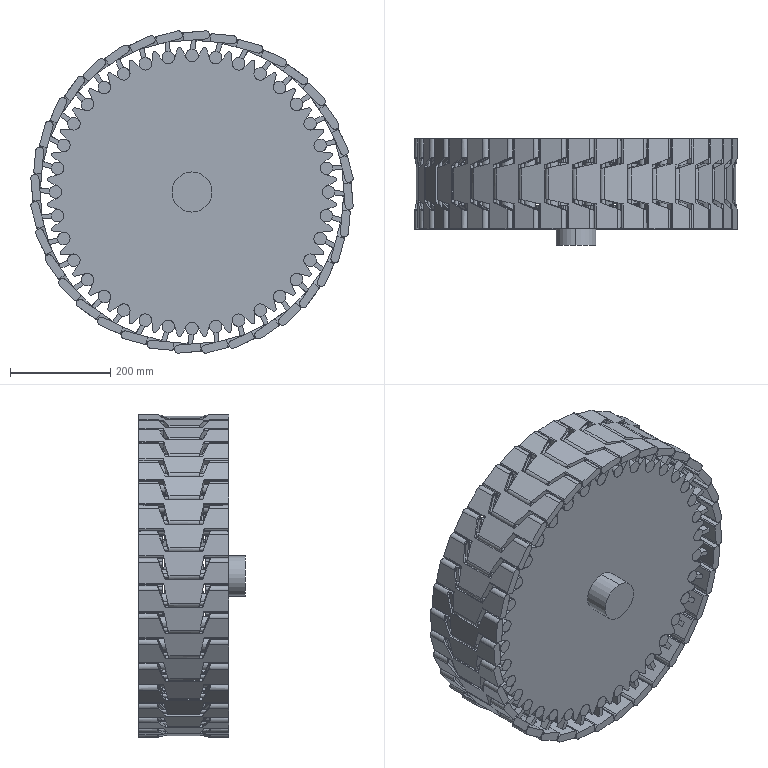Part | SolidWorks | features ReferencePattern 70, CompositeCurve 4, LocalCirPattern 2, RefAxis 1 | 44 solids | 2601 faces | box 643.603 x 212.5 x 643.603 mm | volume 27651397 mm3 | plane 1425 | cylinder 1164 | cone 8 | torus 4 | commonest cylinder face diameters 8 x460 25 x262 16 x216 4 x144 18 x16 20 x16